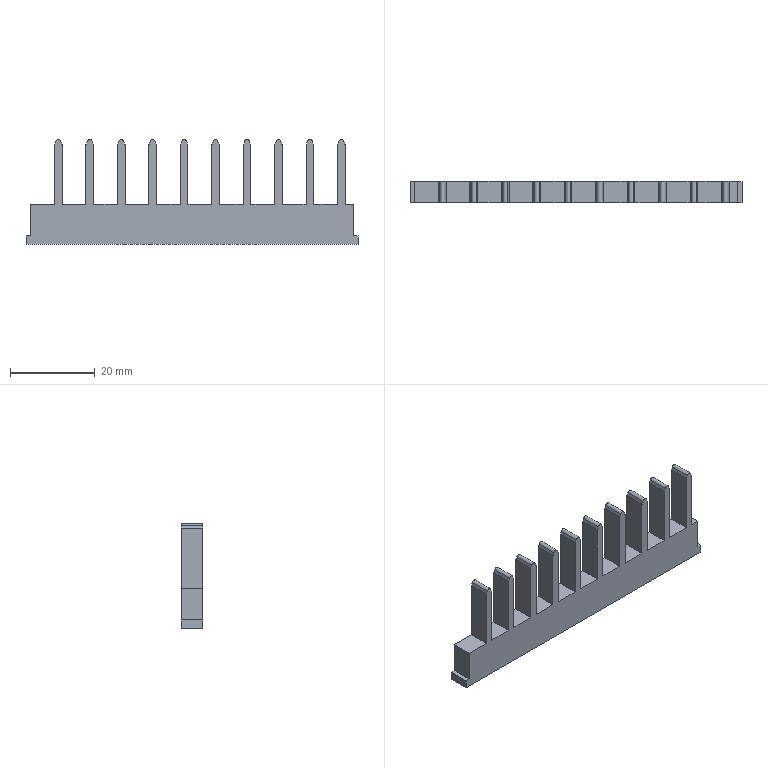Part | STEP file | 200 mesh_id2054 | 1 solid | 90 faces | box 78.34 x 4.98 x 24.75 mm | volume 4951 mm3 | plane 80 | cylinder 10 | commonest cylinder face diameters 1.211 x10